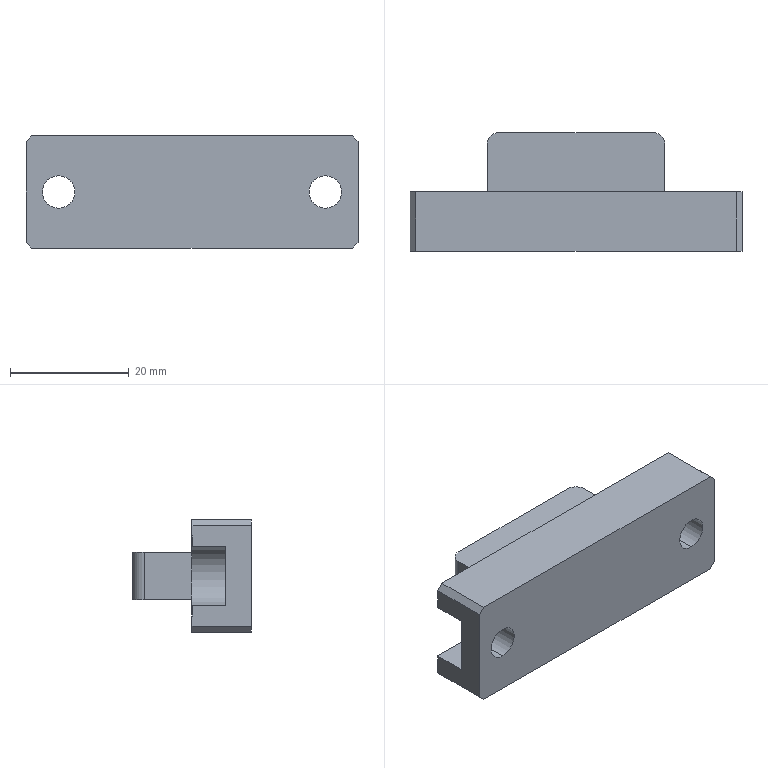Part | SolidWorks | features ICE 2, Chamfer 1, Extrusion 1, Fillet 1, HoleWzd 1 | 1 solid | 29 faces | box 56 x 20 x 19 mm | volume 11727 mm3 | plane 21 | cylinder 8 | commonest cylinder face diameters 5.5 x4 4 x2 10 x2
STEP:
#1=CARTESIAN_POINT('',(-22.5,0.,-2.75));
#2=VERTEX_POINT('',#1);
#3=CARTESIAN_POINT('',(-22.5,0.,2.75));
#4=VERTEX_POINT('',#3);
#5=CARTESIAN_POINT('',(-22.5,0.,0.));
#6=DIRECTION('',(0.,1.,0.));
#7=DIRECTION('',(0.,0.,1.));
#8=AXIS2_PLACEMENT_3D('',#5,#6,#7);
#9=CIRCLE('',#8,2.75);
#10=EDGE_CURVE('',#2,#4,#9,.T.);
#11=ORIENTED_EDGE('',*,*,#10,.F.);
#12=CARTESIAN_POINT('',(-22.5,4.3,-2.75));
#13=VERTEX_POINT('',#12);
#14=CARTESIAN_POINT('',(-22.5,10.,-2.75));
#15=DIRECTION('',(0.,1.,0.));
#16=VECTOR('',#15,1000.);
#17=LINE('',#14,#16);
#18=EDGE_CURVE('',#2,#13,#17,.T.);
#19=ORIENTED_EDGE('',*,*,#18,.T.);
#20=CARTESIAN_POINT('',(-22.5,4.3,2.75));
#21=VERTEX_POINT('',#20);
#22=CARTESIAN_POINT('',(-22.5,4.3,0.));
#23=DIRECTION('',(0.,1.,0.));
#24=DIRECTION('',(0.,0.,1.));
#25=AXIS2_PLACEMENT_3D('',#22,#23,#24);
#26=CIRCLE('',#25,2.75);
#27=EDGE_CURVE('',#13,#21,#26,.T.);
#28=ORIENTED_EDGE('',*,*,#27,.T.);
#29=CARTESIAN_POINT('',(-22.5,10.,2.75));
#30=DIRECTION('',(0.,1.,0.));
#31=VECTOR('',#30,1000.);
#32=LINE('',#29,#31);
#33=EDGE_CURVE('',#4,#21,#32,.T.);
#34=ORIENTED_EDGE('',*,*,#33,.F.);
#35=EDGE_LOOP('',(#11,#19,#28,#34));
#36=FACE_OUTER_BOUND('',#35,.T.);
#37=CARTESIAN_POINT('',(-22.5,10.,0.));
#38=DIRECTION('',(0.,1.,0.));
#39=DIRECTION('',(0.,0.,1.));
#40=AXIS2_PLACEMENT_3D('',#37,#38,#39);
#41=CYLINDRICAL_SURFACE('',#40,2.75);
#42=ADVANCED_FACE('',(#36),#41,.F.);
#43=CARTESIAN_POINT('',(22.5,0.,-2.75));
#44=VERTEX_POINT('',#43);
#45=CARTESIAN_POINT('',(22.5,0.,2.75));
#46=VERTEX_POINT('',#45);
#47=CARTESIAN_POINT('',(22.5,0.,0.));
#48=DIRECTION('',(0.,1.,0.));
#49=DIRECTION('',(0.,0.,1.));
#50=AXIS2_PLACEMENT_3D('',#47,#48,#49);
#51=CIRCLE('',#50,2.75);
#52=EDGE_CURVE('',#44,#46,#51,.T.);
#53=ORIENTED_EDGE('',*,*,#52,.F.);
#54=CARTESIAN_POINT('',(22.5,4.3,-2.75));
#55=VERTEX_POINT('',#54);
#56=CARTESIAN_POINT('',(22.5,10.,-2.75));
#57=DIRECTION('',(0.,1.,0.));
#58=VECTOR('',#57,1000.);
#59=LINE('',#56,#58);
#60=EDGE_CURVE('',#44,#55,#59,.T.);
#61=ORIENTED_EDGE('',*,*,#60,.T.);
#62=CARTESIAN_POINT('',(22.5,4.3,2.75));
#63=VERTEX_POINT('',#62);
#64=CARTESIAN_POINT('',(22.5,4.3,0.));
#65=DIRECTION('',(0.,1.,0.));
#66=DIRECTION('',(0.,0.,1.));
#67=AXIS2_PLACEMENT_3D('',#64,#65,#66);
#68=CIRCLE('',#67,2.75);
#69=EDGE_CURVE('',#55,#63,#68,.T.);
#70=ORIENTED_EDGE('',*,*,#69,.T.);
#71=CARTESIAN_POINT('',(22.5,10.,2.75));
#72=DIRECTION('',(0.,1.,0.));
#73=VECTOR('',#72,1000.);
#74=LINE('',#71,#73);
#75=EDGE_CURVE('',#46,#63,#74,.T.);
#76=ORIENTED_EDGE('',*,*,#75,.F.);
#77=EDGE_LOOP('',(#53,#61,#70,#76));
#78=FACE_OUTER_BOUND('',#77,.T.);
#79=CARTESIAN_POINT('',(22.5,10.,0.));
#80=DIRECTION('',(0.,1.,0.));
#81=DIRECTION('',(0.,0.,1.));
#82=AXIS2_PLACEMENT_3D('',#79,#80,#81);
#83=CYLINDRICAL_SURFACE('',#82,2.75);
#84=ADVANCED_FACE('',(#78),#83,.F.);
#85=CARTESIAN_POINT('',(15.,10.,-4.));
#86=VERTEX_POINT('',#85);
#87=CARTESIAN_POINT('',(15.,18.,-4.));
#88=VERTEX_POINT('',#87);
#89=CARTESIAN_POINT('',(15.,-21.953,-4.));
#90=DIRECTION('',(0.,1.,0.));
#91=VECTOR('',#90,1000.);
#92=LINE('',#89,#91);
#93=EDGE_CURVE('',#86,#88,#92,.T.);
#94=ORIENTED_EDGE('',*,*,#93,.T.);
#95=CARTESIAN_POINT('',(15.,18.,4.));
#96=VERTEX_POINT('',#95);
#97=CARTESIAN_POINT('',(15.,18.,9.5));
#98=DIRECTION('',(0.,0.,1.));
#99=VECTOR('',#98,1000.);
#100=LINE('',#97,#99);
#101=EDGE_CURVE('',#88,#96,#100,.T.);
#102=ORIENTED_EDGE('',*,*,#101,.T.);
#103=CARTESIAN_POINT('',(15.,10.,4.));
#104=VERTEX_POINT('',#103);
#105=CARTESIAN_POINT('',(15.,-21.953,4.));
#106=DIRECTION('',(0.,1.,0.));
#107=VECTOR('',#106,1000.);
#108=LINE('',#105,#107);
#109=EDGE_CURVE('',#104,#96,#108,.T.);
#110=ORIENTED_EDGE('',*,*,#109,.F.);
#111=CARTESIAN_POINT('',(15.,10.,9.5));
#112=DIRECTION('',(0.,0.,-1.));
#113=VECTOR('',#112,1000.);
#114=LINE('',#111,#113);
#115=EDGE_CURVE('',#104,#86,#114,.T.);
#116=ORIENTED_EDGE('',*,*,#115,.T.);
#117=EDGE_LOOP('',(#94,#102,#110,#116));
#118=FACE_OUTER_BOUND('',#117,.T.);
#119=CARTESIAN_POINT('',(15.,10.,9.5));
#120=DIRECTION('',(-1.,0.,0.));
#121=DIRECTION('',(0.,0.,1.));
#122=AXIS2_PLACEMENT_3D('',#119,#120,#121);
#123=PLANE('',#122);
#124=ADVANCED_FACE('',(#118),#123,.F.);
#125=CARTESIAN_POINT('',(13.,20.,4.));
#126=VERTEX_POINT('',#125);
#127=CARTESIAN_POINT('',(-13.,20.,4.));
#128=VERTEX_POINT('',#127);
#129=CARTESIAN_POINT('',(-15.,20.,4.));
#130=DIRECTION('',(-1.,0.,0.));
#131=VECTOR('',#130,1000.);
#132=LINE('',#129,#131);
#133=EDGE_CURVE('',#126,#128,#132,.T.);
#134=ORIENTED_EDGE('',*,*,#133,.F.);
#135=CARTESIAN_POINT('',(13.,20.,-4.));
#136=VERTEX_POINT('',#135);
#137=CARTESIAN_POINT('',(13.,20.,9.5));
#138=DIRECTION('',(0.,0.,-1.));
#139=VECTOR('',#138,1000.);
#140=LINE('',#137,#139);
#141=EDGE_CURVE('',#126,#136,#140,.T.);
#142=ORIENTED_EDGE('',*,*,#141,.T.);
#143=CARTESIAN_POINT('',(-13.,20.,-4.));
#144=VERTEX_POINT('',#143);
#145=CARTESIAN_POINT('',(-15.,20.,-4.));
#146=DIRECTION('',(1.,0.,0.));
#147=VECTOR('',#146,1000.);
#148=LINE('',#145,#147);
#149=EDGE_CURVE('',#144,#136,#148,.T.);
#150=ORIENTED_EDGE('',*,*,#149,.F.);
#151=CARTESIAN_POINT('',(-13.,20.,9.5));
#152=DIRECTION('',(0.,0.,1.));
#153=VECTOR('',#152,1000.);
#154=LINE('',#151,#153);
#155=EDGE_CURVE('',#144,#128,#154,.T.);
#156=ORIENTED_EDGE('',*,*,#155,.T.);
#157=EDGE_LOOP('',(#134,#142,#150,#156));
#158=FACE_OUTER_BOUND('',#157,.T.);
#159=CARTESIAN_POINT('',(-15.,20.,9.5));
#160=DIRECTION('',(0.,-1.,0.));
#161=DIRECTION('',(0.,0.,-1.));
#162=AXIS2_PLACEMENT_3D('',#159,#160,#161);
#163=PLANE('',#162);
#164=ADVANCED_FACE('',(#158),#163,.F.);
#165=CARTESIAN_POINT('',(-15.,10.,4.));
#166=VERTEX_POINT('',#165);
#167=CARTESIAN_POINT('',(-15.,18.,4.));
#168=VERTEX_POINT('',#167);
#169=CARTESIAN_POINT('',(-15.,-21.953,4.));
#170=DIRECTION('',(0.,1.,0.));
#171=VECTOR('',#170,1000.);
#172=LINE('',#169,#171);
#173=EDGE_CURVE('',#166,#168,#172,.T.);
#174=ORIENTED_EDGE('',*,*,#173,.T.);
#175=CARTESIAN_POINT('',(-15.,18.,-4.));
#176=VERTEX_POINT('',#175);
#177=CARTESIAN_POINT('',(-15.,18.,9.5));
#178=DIRECTION('',(0.,0.,-1.));
#179=VECTOR('',#178,1000.);
#180=LINE('',#177,#179);
#181=EDGE_CURVE('',#168,#176,#180,.T.);
#182=ORIENTED_EDGE('',*,*,#181,.T.);
#183=CARTESIAN_POINT('',(-15.,10.,-4.));
#184=VERTEX_POINT('',#183);
#185=CARTESIAN_POINT('',(-15.,-21.953,-4.));
#186=DIRECTION('',(0.,1.,0.));
#187=VECTOR('',#186,1000.);
#188=LINE('',#185,#187);
#189=EDGE_CURVE('',#184,#176,#188,.T.);
#190=ORIENTED_EDGE('',*,*,#189,.F.);
#191=CARTESIAN_POINT('',(-15.,10.,9.5));
#192=DIRECTION('',(0.,0.,-1.));
#193=VECTOR('',#192,1000.);
#194=LINE('',#191,#193);
#195=EDGE_CURVE('',#166,#184,#194,.T.);
#196=ORIENTED_EDGE('',*,*,#195,.F.);
#197=EDGE_LOOP('',(#174,#182,#190,#196));
#198=FACE_OUTER_BOUND('',#197,.T.);
#199=CARTESIAN_POINT('',(-15.,10.,9.5));
#200=DIRECTION('',(1.,0.,0.));
#201=DIRECTION('',(0.,0.,-1.));
#202=AXIS2_PLACEMENT_3D('',#199,#200,#201);
#203=PLANE('',#202);
#204=ADVANCED_FACE('',(#198),#203,.F.);
#205=CARTESIAN_POINT('',(-28.,10.,-5.));
#206=VERTEX_POINT('',#205);
#207=CARTESIAN_POINT('',(-28.,10.,-8.5));
#208=VERTEX_POINT('',#207);
#209=CARTESIAN_POINT('',(-28.,10.,9.5));
#210=DIRECTION('',(0.,0.,-1.));
#211=VECTOR('',#210,1000.);
#212=LINE('',#209,#211);
#213=EDGE_CURVE('',#206,#208,#212,.T.);
#214=ORIENTED_EDGE('',*,*,#213,.T.);
#215=CARTESIAN_POINT('',(-28.,0.,-8.5));
#216=VERTEX_POINT('',#215);
#217=CARTESIAN_POINT('',(-28.,0.,-8.5));
#218=DIRECTION('',(0.,-1.,0.));
#219=VECTOR('',#218,1000.);
#220=LINE('',#217,#219);
#221=EDGE_CURVE('',#208,#216,#220,.T.);
#222=ORIENTED_EDGE('',*,*,#221,.T.);
#223=CARTESIAN_POINT('',(-28.,0.,8.5));
#224=VERTEX_POINT('',#223);
#225=CARTESIAN_POINT('',(-28.,0.,9.5));
#226=DIRECTION('',(0.,0.,-1.));
#227=VECTOR('',#226,1000.);
#228=LINE('',#225,#227);
#229=EDGE_CURVE('',#224,#216,#228,.T.);
#230=ORIENTED_EDGE('',*,*,#229,.F.);
#231=CARTESIAN_POINT('',(-28.,10.,8.5));
#232=VERTEX_POINT('',#231);
#233=CARTESIAN_POINT('',(-28.,0.,8.5));
#234=DIRECTION('',(0.,1.,0.));
#235=VECTOR('',#234,1000.);
#236=LINE('',#233,#235);
#237=EDGE_CURVE('',#224,#232,#236,.T.);
#238=ORIENTED_EDGE('',*,*,#237,.T.);
#239=CARTESIAN_POINT('',(-28.,10.,5.));
#240=VERTEX_POINT('',#239);
#241=CARTESIAN_POINT('',(-28.,10.,9.5));
#242=DIRECTION('',(0.,0.,-1.));
#243=VECTOR('',#242,1000.);
#244=LINE('',#241,#243);
#245=EDGE_CURVE('',#232,#240,#244,.T.);
#246=ORIENTED_EDGE('',*,*,#245,.T.);
#247=CARTESIAN_POINT('',(-28.,4.3,5.));
#248=VERTEX_POINT('',#247);
#249=CARTESIAN_POINT('',(-28.,-7.113,5.));
#250=DIRECTION('',(0.,1.,0.));
#251=VECTOR('',#250,1000.);
#252=LINE('',#249,#251);
#253=EDGE_CURVE('',#248,#240,#252,.T.);
#254=ORIENTED_EDGE('',*,*,#253,.F.);
#255=CARTESIAN_POINT('',(-28.,4.3,-5.));
#256=VERTEX_POINT('',#255);
#257=CARTESIAN_POINT('',(-28.,4.3,5.));
#258=DIRECTION('',(0.,0.,1.));
#259=VECTOR('',#258,1000.);
#260=LINE('',#257,#259);
#261=EDGE_CURVE('',#256,#248,#260,.T.);
#262=ORIENTED_EDGE('',*,*,#261,.F.);
#263=CARTESIAN_POINT('',(-28.,-7.113,-5.));
#264=DIRECTION('',(0.,1.,0.));
#265=VECTOR('',#264,1000.);
#266=LINE('',#263,#265);
#267=EDGE_CURVE('',#256,#206,#266,.T.);
#268=ORIENTED_EDGE('',*,*,#267,.T.);
#269=EDGE_LOOP('',(#214,#222,#230,#238,#246,#254,#262,#268));
#270=FACE_OUTER_BOUND('',#269,.T.);
#271=CARTESIAN_POINT('',(-28.,0.,9.5));
#272=DIRECTION('',(1.,0.,0.));
#273=DIRECTION('',(0.,0.,-1.));
#274=AXIS2_PLACEMENT_3D('',#271,#272,#273);
#275=PLANE('',#274);
#276=ADVANCED_FACE('',(#270),#275,.F.);
#277=CARTESIAN_POINT('',(-22.5,0.,0.));
#278=DIRECTION('',(0.,1.,0.));
#279=DIRECTION('',(0.,0.,1.));
#280=AXIS2_PLACEMENT_3D('',#277,#278,#279);
#281=CIRCLE('',#280,2.75);
#282=EDGE_CURVE('',#4,#2,#281,.T.);
#283=ORIENTED_EDGE('',*,*,#282,.T.);
#284=ORIENTED_EDGE('',*,*,#10,.T.);
#285=EDGE_LOOP('',(#283,#284));
#286=FACE_BOUND('',#285,.T.);
#287=CARTESIAN_POINT('',(22.5,0.,0.));
#288=DIRECTION('',(0.,1.,0.));
#289=DIRECTION('',(0.,0.,1.));
#290=AXIS2_PLACEMENT_3D('',#287,#288,#289);
#291=CIRCLE('',#290,2.75);
#292=EDGE_CURVE('',#46,#44,#291,.T.);
#293=ORIENTED_EDGE('',*,*,#292,.T.);
#294=ORIENTED_EDGE('',*,*,#52,.T.);
#295=EDGE_LOOP('',(#293,#294));
#296=FACE_BOUND('',#295,.T.);
#297=CARTESIAN_POINT('',(28.,0.,8.5));
#298=VERTEX_POINT('',#297);
#299=CARTESIAN_POINT('',(28.,0.,-8.5));
#300=VERTEX_POINT('',#299);
#301=CARTESIAN_POINT('',(28.,0.,9.5));
#302=DIRECTION('',(0.,0.,-1.));
#303=VECTOR('',#302,1000.);
#304=LINE('',#301,#303);
#305=EDGE_CURVE('',#298,#300,#304,.T.);
#306=ORIENTED_EDGE('',*,*,#305,.F.);
#307=CARTESIAN_POINT('',(27.,0.,9.5));
#308=VERTEX_POINT('',#307);
#309=CARTESIAN_POINT('',(27.,0.,9.5));
#310=DIRECTION('',(-0.7071,0.,0.7071));
#311=VECTOR('',#310,1000.);
#312=LINE('',#309,#311);
#313=EDGE_CURVE('',#298,#308,#312,.T.);
#314=ORIENTED_EDGE('',*,*,#313,.T.);
#315=CARTESIAN_POINT('',(-27.,0.,9.5));
#316=VERTEX_POINT('',#315);
#317=CARTESIAN_POINT('',(28.,0.,9.5));
#318=DIRECTION('',(1.,0.,0.));
#319=VECTOR('',#318,1000.);
#320=LINE('',#317,#319);
#321=EDGE_CURVE('',#316,#308,#320,.T.);
#322=ORIENTED_EDGE('',*,*,#321,.F.);
#323=CARTESIAN_POINT('',(-27.,0.,9.5));
#324=DIRECTION('',(-0.7071,0.,-0.7071));
#325=VECTOR('',#324,1000.);
#326=LINE('',#323,#325);
#327=EDGE_CURVE('',#316,#224,#326,.T.);
#328=ORIENTED_EDGE('',*,*,#327,.T.);
#329=ORIENTED_EDGE('',*,*,#229,.T.);
#330=CARTESIAN_POINT('',(-27.,0.,-9.5));
#331=VERTEX_POINT('',#330);
#332=CARTESIAN_POINT('',(-28.,0.,-8.5));
#333=DIRECTION('',(0.7071,0.,-0.7071));
#334=VECTOR('',#333,1000.);
#335=LINE('',#332,#334);
#336=EDGE_CURVE('',#216,#331,#335,.T.);
#337=ORIENTED_EDGE('',*,*,#336,.T.);
#338=CARTESIAN_POINT('',(27.,0.,-9.5));
#339=VERTEX_POINT('',#338);
#340=CARTESIAN_POINT('',(28.,0.,-9.5));
#341=DIRECTION('',(1.,0.,0.));
#342=VECTOR('',#341,1000.);
#343=LINE('',#340,#342);
#344=EDGE_CURVE('',#331,#339,#343,.T.);
#345=ORIENTED_EDGE('',*,*,#344,.T.);
#346=CARTESIAN_POINT('',(28.,0.,-8.5));
#347=DIRECTION('',(0.7071,0.,0.7071));
#348=VECTOR('',#347,1000.);
#349=LINE('',#346,#348);
#350=EDGE_CURVE('',#339,#300,#349,.T.);
#351=ORIENTED_EDGE('',*,*,#350,.T.);
#352=EDGE_LOOP('',(#306,#314,#322,#328,#329,#337,#345,#351));
#353=FACE_OUTER_BOUND('',#352,.T.);
#354=CARTESIAN_POINT('',(28.,0.,9.5));
#355=DIRECTION('',(0.,1.,0.));
#356=DIRECTION('',(0.,0.,1.));
#357=AXIS2_PLACEMENT_3D('',#354,#355,#356);
#358=PLANE('',#357);
#359=ADVANCED_FACE('',(#286,#296,#353),#358,.F.);
#360=CARTESIAN_POINT('',(28.,10.,8.5));
#361=VERTEX_POINT('',#360);
#362=CARTESIAN_POINT('',(28.,10.,5.));
#363=VERTEX_POINT('',#362);
#364=CARTESIAN_POINT('',(28.,10.,9.5));
#365=DIRECTION('',(0.,0.,-1.));
#366=VECTOR('',#365,1000.);
#367=LINE('',#364,#366);
#368=EDGE_CURVE('',#361,#363,#367,.T.);
#369=ORIENTED_EDGE('',*,*,#368,.F.);
#370=CARTESIAN_POINT('',(28.,0.,8.5));
#371=DIRECTION('',(0.,-1.,0.));
#372=VECTOR('',#371,1000.);
#373=LINE('',#370,#372);
#374=EDGE_CURVE('',#361,#298,#373,.T.);
#375=ORIENTED_EDGE('',*,*,#374,.T.);
#376=ORIENTED_EDGE('',*,*,#305,.T.);
#377=CARTESIAN_POINT('',(28.,10.,-8.5));
#378=VERTEX_POINT('',#377);
#379=CARTESIAN_POINT('',(28.,10.,-8.5));
#380=DIRECTION('',(0.,1.,0.));
#381=VECTOR('',#380,1000.);
#382=LINE('',#379,#381);
#383=EDGE_CURVE('',#300,#378,#382,.T.);
#384=ORIENTED_EDGE('',*,*,#383,.T.);
#385=CARTESIAN_POINT('',(28.,10.,-5.));
#386=VERTEX_POINT('',#385);
#387=CARTESIAN_POINT('',(28.,10.,9.5));
#388=DIRECTION('',(0.,0.,-1.));
#389=VECTOR('',#388,1000.);
#390=LINE('',#387,#389);
#391=EDGE_CURVE('',#386,#378,#390,.T.);
#392=ORIENTED_EDGE('',*,*,#391,.F.);
#393=CARTESIAN_POINT('',(28.,4.3,-5.));
#394=VERTEX_POINT('',#393);
#395=CARTESIAN_POINT('',(28.,-7.113,-5.));
#396=DIRECTION('',(0.,1.,0.));
#397=VECTOR('',#396,1000.);
#398=LINE('',#395,#397);
#399=EDGE_CURVE('',#394,#386,#398,.T.);
#400=ORIENTED_EDGE('',*,*,#399,.F.);
#401=CARTESIAN_POINT('',(28.,4.3,5.));
#402=VERTEX_POINT('',#401);
#403=CARTESIAN_POINT('',(28.,4.3,5.));
#404=DIRECTION('',(0.,0.,-1.));
#405=VECTOR('',#404,1000.);
#406=LINE('',#403,#405);
#407=EDGE_CURVE('',#402,#394,#406,.T.);
#408=ORIENTED_EDGE('',*,*,#407,.F.);
#409=CARTESIAN_POINT('',(28.,-7.113,5.));
#410=DIRECTION('',(0.,1.,0.));
#411=VECTOR('',#410,1000.);
#412=LINE('',#409,#411);
#413=EDGE_CURVE('',#402,#363,#412,.T.);
#414=ORIENTED_EDGE('',*,*,#413,.T.);
#415=EDGE_LOOP('',(#369,#375,#376,#384,#392,#400,#408,#414));
#416=FACE_OUTER_BOUND('',#415,.T.);
#417=CARTESIAN_POINT('',(28.,0.,9.5));
#418=DIRECTION('',(-1.,0.,0.));
#419=DIRECTION('',(0.,0.,1.));
#420=AXIS2_PLACEMENT_3D('',#417,#418,#419);
#421=PLANE('',#420);
#422=ADVANCED_FACE('',(#416),#421,.F.);
#423=CARTESIAN_POINT('',(-15.,10.,4.));
#424=DIRECTION('',(-1.,0.,0.));
#425=VECTOR('',#424,1000.);
#426=LINE('',#423,#425);
#427=EDGE_CURVE('',#104,#166,#426,.T.);
#428=ORIENTED_EDGE('',*,*,#427,.T.);
#429=ORIENTED_EDGE('',*,*,#195,.T.);
#430=CARTESIAN_POINT('',(-15.,10.,-4.));
#431=DIRECTION('',(1.,0.,0.));
#432=VECTOR('',#431,1000.);
#433=LINE('',#430,#432);
#434=EDGE_CURVE('',#184,#86,#433,.T.);
#435=ORIENTED_EDGE('',*,*,#434,.T.);
#436=ORIENTED_EDGE('',*,*,#115,.F.);
#437=EDGE_LOOP('',(#428,#429,#435,#436));
#438=FACE_BOUND('',#437,.T.);
#439=CARTESIAN_POINT('',(27.,10.,9.5));
#440=VERTEX_POINT('',#439);
#441=CARTESIAN_POINT('',(-27.,10.,9.5));
#442=VERTEX_POINT('',#441);
#443=CARTESIAN_POINT('',(-28.,10.,9.5));
#444=DIRECTION('',(-1.,0.,0.));
#445=VECTOR('',#444,1000.);
#446=LINE('',#443,#445);
#447=EDGE_CURVE('',#440,#442,#446,.T.);
#448=ORIENTED_EDGE('',*,*,#447,.F.);
#449=CARTESIAN_POINT('',(27.,10.,9.5));
#450=DIRECTION('',(0.7071,0.,-0.7071));
#451=VECTOR('',#450,1000.);
#452=LINE('',#449,#451);
#453=EDGE_CURVE('',#440,#361,#452,.T.);
#454=ORIENTED_EDGE('',*,*,#453,.T.);
#455=ORIENTED_EDGE('',*,*,#368,.T.);
#456=CARTESIAN_POINT('',(22.5,10.,5.));
#457=VERTEX_POINT('',#456);
#458=CARTESIAN_POINT('',(22.5,10.,5.));
#459=DIRECTION('',(1.,0.,0.));
#460=VECTOR('',#459,1000.);
#461=LINE('',#458,#460);
#462=EDGE_CURVE('',#457,#363,#461,.T.);
#463=ORIENTED_EDGE('',*,*,#462,.F.);
#464=CARTESIAN_POINT('',(22.5,10.,-5.));
#465=VERTEX_POINT('',#464);
#466=CARTESIAN_POINT('',(22.5,10.,0.));
#467=DIRECTION('',(0.,1.,0.));
#468=DIRECTION('',(0.,0.,1.));
#469=AXIS2_PLACEMENT_3D('',#466,#467,#468);
#470=CIRCLE('',#469,5.);
#471=EDGE_CURVE('',#465,#457,#470,.T.);
#472=ORIENTED_EDGE('',*,*,#471,.F.);
#473=CARTESIAN_POINT('',(22.5,10.,-5.));
#474=DIRECTION('',(-1.,0.,0.));
#475=VECTOR('',#474,1000.);
#476=LINE('',#473,#475);
#477=EDGE_CURVE('',#386,#465,#476,.T.);
#478=ORIENTED_EDGE('',*,*,#477,.F.);
#479=ORIENTED_EDGE('',*,*,#391,.T.);
#480=CARTESIAN_POINT('',(27.,10.,-9.5));
#481=VERTEX_POINT('',#480);
#482=CARTESIAN_POINT('',(28.,10.,-8.5));
#483=DIRECTION('',(-0.7071,0.,-0.7071));
#484=VECTOR('',#483,1000.);
#485=LINE('',#482,#484);
#486=EDGE_CURVE('',#378,#481,#485,.T.);
#487=ORIENTED_EDGE('',*,*,#486,.T.);
#488=CARTESIAN_POINT('',(-27.,10.,-9.5));
#489=VERTEX_POINT('',#488);
#490=CARTESIAN_POINT('',(28.,10.,-9.5));
#491=DIRECTION('',(-1.,0.,0.));
#492=VECTOR('',#491,1000.);
#493=LINE('',#490,#492);
#494=EDGE_CURVE('',#481,#489,#493,.T.);
#495=ORIENTED_EDGE('',*,*,#494,.T.);
#496=CARTESIAN_POINT('',(-28.,10.,-8.5));
#497=DIRECTION('',(-0.7071,0.,0.7071));
#498=VECTOR('',#497,1000.);
#499=LINE('',#496,#498);
#500=EDGE_CURVE('',#489,#208,#499,.T.);
#501=ORIENTED_EDGE('',*,*,#500,.T.);
#502=ORIENTED_EDGE('',*,*,#213,.F.);
#503=CARTESIAN_POINT('',(-22.5,10.,-5.));
#504=VERTEX_POINT('',#503);
#505=CARTESIAN_POINT('',(-28.,10.,-5.));
#506=DIRECTION('',(-1.,0.,0.));
#507=VECTOR('',#506,1000.);
#508=LINE('',#505,#507);
#509=EDGE_CURVE('',#504,#206,#508,.T.);
#510=ORIENTED_EDGE('',*,*,#509,.F.);
#511=CARTESIAN_POINT('',(-22.5,10.,5.));
#512=VERTEX_POINT('',#511);
#513=CARTESIAN_POINT('',(-22.5,10.,0.));
#514=DIRECTION('',(0.,1.,0.));
#515=DIRECTION('',(0.,0.,1.));
#516=AXIS2_PLACEMENT_3D('',#513,#514,#515);
#517=CIRCLE('',#516,5.);
#518=EDGE_CURVE('',#512,#504,#517,.T.);
#519=ORIENTED_EDGE('',*,*,#518,.F.);
#520=CARTESIAN_POINT('',(-28.,10.,5.));
#521=DIRECTION('',(1.,0.,0.));
#522=VECTOR('',#521,1000.);
#523=LINE('',#520,#522);
#524=EDGE_CURVE('',#240,#512,#523,.T.);
#525=ORIENTED_EDGE('',*,*,#524,.F.);
#526=ORIENTED_EDGE('',*,*,#245,.F.);
#527=CARTESIAN_POINT('',(-27.,10.,9.5));
#528=DIRECTION('',(0.7071,0.,0.7071));
#529=VECTOR('',#528,1000.);
#530=LINE('',#527,#529);
#531=EDGE_CURVE('',#232,#442,#530,.T.);
#532=ORIENTED_EDGE('',*,*,#531,.T.);
#533=EDGE_LOOP('',(#448,#454,#455,#463,#472,#478,#479,#487,#495,#501,#502,#510,#519,#525,#526,#532));
#534=FACE_OUTER_BOUND('',#533,.T.);
#535=CARTESIAN_POINT('',(28.,10.,9.5));
#536=DIRECTION('',(0.,-1.,0.));
#537=DIRECTION('',(1.,0.,0.));
#538=AXIS2_PLACEMENT_3D('',#535,#536,#537);
#539=PLANE('',#538);
#540=ADVANCED_FACE('',(#438,#534),#539,.F.);
#541=ORIENTED_EDGE('',*,*,#321,.T.);
#542=CARTESIAN_POINT('',(27.,20.,9.5));
#543=DIRECTION('',(0.,1.,0.));
#544=VECTOR('',#543,1000.);
#545=LINE('',#542,#544);
#546=EDGE_CURVE('',#308,#440,#545,.T.);
#547=ORIENTED_EDGE('',*,*,#546,.T.);
#548=ORIENTED_EDGE('',*,*,#447,.T.);
#549=CARTESIAN_POINT('',(-27.,20.,9.5));
#550=DIRECTION('',(0.,-1.,0.));
#551=VECTOR('',#550,1000.);
#552=LINE('',#549,#551);
#553=EDGE_CURVE('',#442,#316,#552,.T.);
#554=ORIENTED_EDGE('',*,*,#553,.T.);
#555=EDGE_LOOP('',(#541,#547,#548,#554));
#556=FACE_OUTER_BOUND('',#555,.T.);
#557=CARTESIAN_POINT('',(15.,20.,9.5));
#558=DIRECTION('',(0.,0.,-1.));
#559=DIRECTION('',(-1.,0.,0.));
#560=AXIS2_PLACEMENT_3D('',#557,#558,#559);
#561=PLANE('',#560);
#562=ADVANCED_FACE('',(#556),#561,.F.);
#563=ORIENTED_EDGE('',*,*,#494,.F.);
#564=CARTESIAN_POINT('',(27.,0.,-9.5));
#565=DIRECTION('',(0.,-1.,0.));
#566=VECTOR('',#565,1000.);
#567=LINE('',#564,#566);
#568=EDGE_CURVE('',#481,#339,#567,.T.);
#569=ORIENTED_EDGE('',*,*,#568,.T.);
#570=ORIENTED_EDGE('',*,*,#344,.F.);
#571=CARTESIAN_POINT('',(-27.,10.,-9.5));
#572=DIRECTION('',(0.,1.,0.));
#573=VECTOR('',#572,1000.);
#574=LINE('',#571,#573);
#575=EDGE_CURVE('',#331,#489,#574,.T.);
#576=ORIENTED_EDGE('',*,*,#575,.T.);
#577=EDGE_LOOP('',(#563,#569,#570,#576));
#578=FACE_OUTER_BOUND('',#577,.T.);
#579=CARTESIAN_POINT('',(15.,20.,-9.5));
#580=DIRECTION('',(0.,0.,-1.));
#581=DIRECTION('',(-1.,0.,0.));
#582=AXIS2_PLACEMENT_3D('',#579,#580,#581);
#583=PLANE('',#582);
#584=ADVANCED_FACE('',(#578),#583,.T.);
#585=ORIENTED_EDGE('',*,*,#60,.F.);
#586=ORIENTED_EDGE('',*,*,#292,.F.);
#587=ORIENTED_EDGE('',*,*,#75,.T.);
#588=CARTESIAN_POINT('',(22.5,4.3,0.));
#589=DIRECTION('',(0.,1.,0.));
#590=DIRECTION('',(0.,0.,1.));
#591=AXIS2_PLACEMENT_3D('',#588,#589,#590);
#592=CIRCLE('',#591,2.75);
#593=EDGE_CURVE('',#63,#55,#592,.T.);
#594=ORIENTED_EDGE('',*,*,#593,.T.);
#595=EDGE_LOOP('',(#585,#586,#587,#594));
#596=FACE_OUTER_BOUND('',#595,.T.);
#597=CARTESIAN_POINT('',(22.5,10.,0.));
#598=DIRECTION('',(0.,1.,0.));
#599=DIRECTION('',(0.,0.,1.));
#600=AXIS2_PLACEMENT_3D('',#597,#598,#599);
#601=CYLINDRICAL_SURFACE('',#600,2.75);
#602=ADVANCED_FACE('',(#596),#601,.F.);
#603=ORIENTED_EDGE('',*,*,#593,.F.);
#604=ORIENTED_EDGE('',*,*,#69,.F.);
#605=EDGE_LOOP('',(#603,#604));
#606=FACE_BOUND('',#605,.T.);
#607=CARTESIAN_POINT('',(22.5,4.3,-5.));
#608=VERTEX_POINT('',#607);
#609=CARTESIAN_POINT('',(22.5,4.3,5.));
#610=VERTEX_POINT('',#609);
#611=CARTESIAN_POINT('',(22.5,4.3,0.));
#612=DIRECTION('',(0.,1.,0.));
#613=DIRECTION('',(0.,0.,1.));
#614=AXIS2_PLACEMENT_3D('',#611,#612,#613);
#615=CIRCLE('',#614,5.);
#616=EDGE_CURVE('',#608,#610,#615,.T.);
#617=ORIENTED_EDGE('',*,*,#616,.T.);
#618=CARTESIAN_POINT('',(22.5,4.3,5.));
#619=DIRECTION('',(1.,0.,0.));
#620=VECTOR('',#619,1000.);
#621=LINE('',#618,#620);
#622=EDGE_CURVE('',#610,#402,#621,.T.);
#623=ORIENTED_EDGE('',*,*,#622,.T.);
#624=ORIENTED_EDGE('',*,*,#407,.T.);
#625=CARTESIAN_POINT('',(22.5,4.3,-5.));
#626=DIRECTION('',(-1.,0.,0.));
#627=VECTOR('',#626,1000.);
#628=LINE('',#625,#627);
#629=EDGE_CURVE('',#394,#608,#628,.T.);
#630=ORIENTED_EDGE('',*,*,#629,.T.);
#631=EDGE_LOOP('',(#617,#623,#624,#630));
#632=FACE_OUTER_BOUND('',#631,.T.);
#633=CARTESIAN_POINT('',(25.25,4.3,0.));
#634=DIRECTION('',(0.,-1.,0.));
#635=DIRECTION('',(0.,0.,-1.));
#636=AXIS2_PLACEMENT_3D('',#633,#634,#635);
#637=PLANE('',#636);
#638=ADVANCED_FACE('',(#606,#632),#637,.F.);
#639=ORIENTED_EDGE('',*,*,#471,.T.);
#640=CARTESIAN_POINT('',(22.5,-7.113,5.));
#641=DIRECTION('',(0.,1.,0.));
#642=VECTOR('',#641,1000.);
#643=LINE('',#640,#642);
#644=EDGE_CURVE('',#610,#457,#643,.T.);
#645=ORIENTED_EDGE('',*,*,#644,.F.);
#646=ORIENTED_EDGE('',*,*,#616,.F.);
#647=CARTESIAN_POINT('',(22.5,-7.113,-5.));
#648=DIRECTION('',(0.,1.,0.));
#649=VECTOR('',#648,1000.);
#650=LINE('',#647,#649);
#651=EDGE_CURVE('',#608,#465,#650,.T.);
#652=ORIENTED_EDGE('',*,*,#651,.T.);
#653=EDGE_LOOP('',(#639,#645,#646,#652));
#654=FACE_OUTER_BOUND('',#653,.T.);
#655=CARTESIAN_POINT('',(22.5,10.,0.));
#656=DIRECTION('',(0.,1.,0.));
#657=DIRECTION('',(0.,0.,1.));
#658=AXIS2_PLACEMENT_3D('',#655,#656,#657);
#659=CYLINDRICAL_SURFACE('',#658,5.);
#660=ADVANCED_FACE('',(#654),#659,.F.);
#661=ORIENTED_EDGE('',*,*,#18,.F.);
#662=ORIENTED_EDGE('',*,*,#282,.F.);
#663=ORIENTED_EDGE('',*,*,#33,.T.);
#664=CARTESIAN_POINT('',(-22.5,4.3,0.));
#665=DIRECTION('',(0.,1.,0.));
#666=DIRECTION('',(0.,0.,1.));
#667=AXIS2_PLACEMENT_3D('',#664,#665,#666);
#668=CIRCLE('',#667,2.75);
#669=EDGE_CURVE('',#21,#13,#668,.T.);
#670=ORIENTED_EDGE('',*,*,#669,.T.);
#671=EDGE_LOOP('',(#661,#662,#663,#670));
#672=FACE_OUTER_BOUND('',#671,.T.);
#673=CARTESIAN_POINT('',(-22.5,10.,0.));
#674=DIRECTION('',(0.,1.,0.));
#675=DIRECTION('',(0.,0.,1.));
#676=AXIS2_PLACEMENT_3D('',#673,#674,#675);
#677=CYLINDRICAL_SURFACE('',#676,2.75);
#678=ADVANCED_FACE('',(#672),#677,.F.);
#679=ORIENTED_EDGE('',*,*,#669,.F.);
#680=ORIENTED_EDGE('',*,*,#27,.F.);
#681=EDGE_LOOP('',(#679,#680));
#682=FACE_BOUND('',#681,.T.);
#683=CARTESIAN_POINT('',(-22.5,4.3,5.));
#684=VERTEX_POINT('',#683);
#685=CARTESIAN_POINT('',(-22.5,4.3,-5.));
#686=VERTEX_POINT('',#685);
#687=CARTESIAN_POINT('',(-22.5,4.3,0.));
#688=DIRECTION('',(0.,1.,0.));
#689=DIRECTION('',(0.,0.,1.));
#690=AXIS2_PLACEMENT_3D('',#687,#688,#689);
#691=CIRCLE('',#690,5.);
#692=EDGE_CURVE('',#684,#686,#691,.T.);
#693=ORIENTED_EDGE('',*,*,#692,.T.);
#694=CARTESIAN_POINT('',(-28.,4.3,-5.));
#695=DIRECTION('',(-1.,0.,0.));
#696=VECTOR('',#695,1000.);
#697=LINE('',#694,#696);
#698=EDGE_CURVE('',#686,#256,#697,.T.);
#699=ORIENTED_EDGE('',*,*,#698,.T.);
#700=ORIENTED_EDGE('',*,*,#261,.T.);
#701=CARTESIAN_POINT('',(-28.,4.3,5.));
#702=DIRECTION('',(1.,0.,0.));
#703=VECTOR('',#702,1000.);
#704=LINE('',#701,#703);
#705=EDGE_CURVE('',#248,#684,#704,.T.);
#706=ORIENTED_EDGE('',*,*,#705,.T.);
#707=EDGE_LOOP('',(#693,#699,#700,#706));
#708=FACE_OUTER_BOUND('',#707,.T.);
#709=CARTESIAN_POINT('',(-19.75,4.3,0.));
#710=DIRECTION('',(0.,-1.,0.));
#711=DIRECTION('',(0.,0.,-1.));
#712=AXIS2_PLACEMENT_3D('',#709,#710,#711);
#713=PLANE('',#712);
#714=ADVANCED_FACE('',(#682,#708),#713,.F.);
#715=ORIENTED_EDGE('',*,*,#692,.F.);
#716=CARTESIAN_POINT('',(-22.5,-7.113,5.));
#717=DIRECTION('',(0.,1.,0.));
#718=VECTOR('',#717,1000.);
#719=LINE('',#716,#718);
#720=EDGE_CURVE('',#684,#512,#719,.T.);
#721=ORIENTED_EDGE('',*,*,#720,.T.);
#722=ORIENTED_EDGE('',*,*,#518,.T.);
#723=CARTESIAN_POINT('',(-22.5,-7.113,-5.));
#724=DIRECTION('',(0.,1.,0.));
#725=VECTOR('',#724,1000.);
#726=LINE('',#723,#725);
#727=EDGE_CURVE('',#686,#504,#726,.T.);
#728=ORIENTED_EDGE('',*,*,#727,.F.);
#729=EDGE_LOOP('',(#715,#721,#722,#728));
#730=FACE_OUTER_BOUND('',#729,.T.);
#731=CARTESIAN_POINT('',(-22.5,10.,0.));
#732=DIRECTION('',(0.,1.,0.));
#733=DIRECTION('',(0.,0.,1.));
#734=AXIS2_PLACEMENT_3D('',#731,#732,#733);
#735=CYLINDRICAL_SURFACE('',#734,5.);
#736=ADVANCED_FACE('',(#730),#735,.F.);
#737=ORIENTED_EDGE('',*,*,#253,.T.);
#738=ORIENTED_EDGE('',*,*,#524,.T.);
#739=ORIENTED_EDGE('',*,*,#720,.F.);
#740=ORIENTED_EDGE('',*,*,#705,.F.);
#741=EDGE_LOOP('',(#737,#738,#739,#740));
#742=FACE_OUTER_BOUND('',#741,.T.);
#743=CARTESIAN_POINT('',(-28.,-7.113,5.));
#744=DIRECTION('',(0.,0.,1.));
#745=DIRECTION('',(1.,0.,0.));
#746=AXIS2_PLACEMENT_3D('',#743,#744,#745);
#747=PLANE('',#746);
#748=ADVANCED_FACE('',(#742),#747,.F.);
#749=ORIENTED_EDGE('',*,*,#727,.T.);
#750=ORIENTED_EDGE('',*,*,#509,.T.);
#751=ORIENTED_EDGE('',*,*,#267,.F.);
#752=ORIENTED_EDGE('',*,*,#698,.F.);
#753=EDGE_LOOP('',(#749,#750,#751,#752));
#754=FACE_OUTER_BOUND('',#753,.T.);
#755=CARTESIAN_POINT('',(-28.,-7.113,-5.));
#756=DIRECTION('',(0.,0.,-1.));
#757=DIRECTION('',(-1.,0.,0.));
#758=AXIS2_PLACEMENT_3D('',#755,#756,#757);
#759=PLANE('',#758);
#760=ADVANCED_FACE('',(#754),#759,.F.);
#761=ORIENTED_EDGE('',*,*,#644,.T.);
#762=ORIENTED_EDGE('',*,*,#462,.T.);
#763=ORIENTED_EDGE('',*,*,#413,.F.);
#764=ORIENTED_EDGE('',*,*,#622,.F.);
#765=EDGE_LOOP('',(#761,#762,#763,#764));
#766=FACE_OUTER_BOUND('',#765,.T.);
#767=CARTESIAN_POINT('',(22.5,-7.113,5.));
#768=DIRECTION('',(0.,0.,1.));
#769=DIRECTION('',(1.,0.,0.));
#770=AXIS2_PLACEMENT_3D('',#767,#768,#769);
#771=PLANE('',#770);
#772=ADVANCED_FACE('',(#766),#771,.F.);
#773=ORIENTED_EDGE('',*,*,#399,.T.);
#774=ORIENTED_EDGE('',*,*,#477,.T.);
#775=ORIENTED_EDGE('',*,*,#651,.F.);
#776=ORIENTED_EDGE('',*,*,#629,.F.);
#777=EDGE_LOOP('',(#773,#774,#775,#776));
#778=FACE_OUTER_BOUND('',#777,.T.);
#779=CARTESIAN_POINT('',(22.5,-7.113,-5.));
#780=DIRECTION('',(0.,0.,-1.));
#781=DIRECTION('',(-1.,0.,0.));
#782=AXIS2_PLACEMENT_3D('',#779,#780,#781);
#783=PLANE('',#782);
#784=ADVANCED_FACE('',(#778),#783,.F.);
#785=ORIENTED_EDGE('',*,*,#149,.T.);
#786=CARTESIAN_POINT('',(13.,18.,-4.));
#787=DIRECTION('',(0.,0.,-1.));
#788=DIRECTION('',(1.,0.,0.));
#789=AXIS2_PLACEMENT_3D('',#786,#787,#788);
#790=CIRCLE('',#789,2.);
#791=EDGE_CURVE('',#136,#88,#790,.T.);
#792=ORIENTED_EDGE('',*,*,#791,.T.);
#793=ORIENTED_EDGE('',*,*,#93,.F.);
#794=ORIENTED_EDGE('',*,*,#434,.F.);
#795=ORIENTED_EDGE('',*,*,#189,.T.);
#796=CARTESIAN_POINT('',(-13.,18.,-4.));
#797=DIRECTION('',(0.,0.,-1.));
#798=DIRECTION('',(1.,0.,0.));
#799=AXIS2_PLACEMENT_3D('',#796,#797,#798);
#800=CIRCLE('',#799,2.);
#801=EDGE_CURVE('',#176,#144,#800,.T.);
#802=ORIENTED_EDGE('',*,*,#801,.T.);
#803=EDGE_LOOP('',(#785,#792,#793,#794,#795,#802));
#804=FACE_OUTER_BOUND('',#803,.T.);
#805=CARTESIAN_POINT('',(-15.,-21.953,-4.));
#806=DIRECTION('',(0.,0.,1.));
#807=DIRECTION('',(1.,0.,0.));
#808=AXIS2_PLACEMENT_3D('',#805,#806,#807);
#809=PLANE('',#808);
#810=ADVANCED_FACE('',(#804),#809,.F.);
#811=ORIENTED_EDGE('',*,*,#109,.T.);
#812=CARTESIAN_POINT('',(13.,18.,4.));
#813=DIRECTION('',(0.,0.,1.));
#814=DIRECTION('',(-1.,0.,0.));
#815=AXIS2_PLACEMENT_3D('',#812,#813,#814);
#816=CIRCLE('',#815,2.);
#817=EDGE_CURVE('',#96,#126,#816,.T.);
#818=ORIENTED_EDGE('',*,*,#817,.T.);
#819=ORIENTED_EDGE('',*,*,#133,.T.);
#820=CARTESIAN_POINT('',(-13.,18.,4.));
#821=DIRECTION('',(0.,0.,1.));
#822=DIRECTION('',(-1.,0.,0.));
#823=AXIS2_PLACEMENT_3D('',#820,#821,#822);
#824=CIRCLE('',#823,2.);
#825=EDGE_CURVE('',#128,#168,#824,.T.);
#826=ORIENTED_EDGE('',*,*,#825,.T.);
#827=ORIENTED_EDGE('',*,*,#173,.F.);
#828=ORIENTED_EDGE('',*,*,#427,.F.);
#829=EDGE_LOOP('',(#811,#818,#819,#826,#827,#828));
#830=FACE_OUTER_BOUND('',#829,.T.);
#831=CARTESIAN_POINT('',(-15.,-21.953,4.));
#832=DIRECTION('',(0.,0.,-1.));
#833=DIRECTION('',(-1.,0.,0.));
#834=AXIS2_PLACEMENT_3D('',#831,#832,#833);
#835=PLANE('',#834);
#836=ADVANCED_FACE('',(#830),#835,.F.);
#837=ORIENTED_EDGE('',*,*,#313,.F.);
#838=ORIENTED_EDGE('',*,*,#374,.F.);
#839=ORIENTED_EDGE('',*,*,#453,.F.);
#840=ORIENTED_EDGE('',*,*,#546,.F.);
#841=EDGE_LOOP('',(#837,#838,#839,#840));
#842=FACE_OUTER_BOUND('',#841,.T.);
#843=CARTESIAN_POINT('',(27.,20.,9.5));
#844=DIRECTION('',(-0.7071,0.,-0.7071));
#845=DIRECTION('',(-0.7071,0.,0.7071));
#846=AXIS2_PLACEMENT_3D('',#843,#844,#845);
#847=PLANE('',#846);
#848=ADVANCED_FACE('',(#842),#847,.F.);
#849=ORIENTED_EDGE('',*,*,#350,.F.);
#850=ORIENTED_EDGE('',*,*,#568,.F.);
#851=ORIENTED_EDGE('',*,*,#486,.F.);
#852=ORIENTED_EDGE('',*,*,#383,.F.);
#853=EDGE_LOOP('',(#849,#850,#851,#852));
#854=FACE_OUTER_BOUND('',#853,.T.);
#855=CARTESIAN_POINT('',(28.,0.,-8.5));
#856=DIRECTION('',(0.7071,0.,-0.7071));
#857=DIRECTION('',(-0.7071,0.,-0.7071));
#858=AXIS2_PLACEMENT_3D('',#855,#856,#857);
#859=PLANE('',#858);
#860=ADVANCED_FACE('',(#854),#859,.T.);
#861=ORIENTED_EDGE('',*,*,#500,.F.);
#862=ORIENTED_EDGE('',*,*,#575,.F.);
#863=ORIENTED_EDGE('',*,*,#336,.F.);
#864=ORIENTED_EDGE('',*,*,#221,.F.);
#865=EDGE_LOOP('',(#861,#862,#863,#864));
#866=FACE_OUTER_BOUND('',#865,.T.);
#867=CARTESIAN_POINT('',(-28.,0.,-8.5));
#868=DIRECTION('',(-0.7071,0.,-0.7071));
#869=DIRECTION('',(-0.7071,0.,0.7071));
#870=AXIS2_PLACEMENT_3D('',#867,#868,#869);
#871=PLANE('',#870);
#872=ADVANCED_FACE('',(#866),#871,.T.);
#873=ORIENTED_EDGE('',*,*,#531,.F.);
#874=ORIENTED_EDGE('',*,*,#237,.F.);
#875=ORIENTED_EDGE('',*,*,#327,.F.);
#876=ORIENTED_EDGE('',*,*,#553,.F.);
#877=EDGE_LOOP('',(#873,#874,#875,#876));
#878=FACE_OUTER_BOUND('',#877,.T.);
#879=CARTESIAN_POINT('',(-27.,20.,9.5));
#880=DIRECTION('',(0.7071,0.,-0.7071));
#881=DIRECTION('',(-0.7071,0.,-0.7071));
#882=AXIS2_PLACEMENT_3D('',#879,#880,#881);
#883=PLANE('',#882);
#884=ADVANCED_FACE('',(#878),#883,.F.);
#885=ORIENTED_EDGE('',*,*,#817,.F.);
#886=ORIENTED_EDGE('',*,*,#101,.F.);
#887=ORIENTED_EDGE('',*,*,#791,.F.);
#888=ORIENTED_EDGE('',*,*,#141,.F.);
#889=EDGE_LOOP('',(#885,#886,#887,#888));
#890=FACE_OUTER_BOUND('',#889,.T.);
#891=CARTESIAN_POINT('',(13.,18.,9.5));
#892=DIRECTION('',(0.,0.,-1.));
#893=DIRECTION('',(-1.,0.,0.));
#894=AXIS2_PLACEMENT_3D('',#891,#892,#893);
#895=CYLINDRICAL_SURFACE('',#894,2.);
#896=ADVANCED_FACE('',(#890),#895,.T.);
#897=ORIENTED_EDGE('',*,*,#825,.F.);
#898=ORIENTED_EDGE('',*,*,#155,.F.);
#899=ORIENTED_EDGE('',*,*,#801,.F.);
#900=ORIENTED_EDGE('',*,*,#181,.F.);
#901=EDGE_LOOP('',(#897,#898,#899,#900));
#902=FACE_OUTER_BOUND('',#901,.T.);
#903=CARTESIAN_POINT('',(-13.,18.,9.5));
#904=DIRECTION('',(0.,0.,-1.));
#905=DIRECTION('',(-1.,0.,0.));
#906=AXIS2_PLACEMENT_3D('',#903,#904,#905);
#907=CYLINDRICAL_SURFACE('',#906,2.);
#908=ADVANCED_FACE('',(#902),#907,.T.);
#909=CLOSED_SHELL('',(#42,#84,#124,#164,#204,#276,#359,#422,#540,#562,#584,#602,#638,#660,#678,#714,#736,#748,#760,#772,#784,#810,#836,#848,#860,#872,#884,#896,#908));
#910=MANIFOLD_SOLID_BREP('',#909);
#911=CARTESIAN_POINT('',(0.,0.,0.));
#912=DIRECTION('',(0.,0.,1.));
#913=DIRECTION('',(1.,0.,0.));
#914=AXIS2_PLACEMENT_3D('',#911,#912,#913);
#915=(LENGTH_UNIT()NAMED_UNIT(*)SI_UNIT(.MILLI.,.METRE.));
#916=UNCERTAINTY_MEASURE_WITH_UNIT(LENGTH_MEASURE(0.00001),#915,'','');
#917=(NAMED_UNIT(*)PLANE_ANGLE_UNIT()SI_UNIT($,.RADIAN.));
#918=(NAMED_UNIT(*)SI_UNIT($,.STERADIAN.)SOLID_ANGLE_UNIT());
#919=(GEOMETRIC_REPRESENTATION_CONTEXT(3)GLOBAL_UNCERTAINTY_ASSIGNED_CONTEXT((#916))GLOBAL_UNIT_ASSIGNED_CONTEXT((#915,#917,#918))REPRESENTATION_CONTEXT('',''));
#920=ADVANCED_BREP_SHAPE_REPRESENTATION('',(#910,#914),#919);